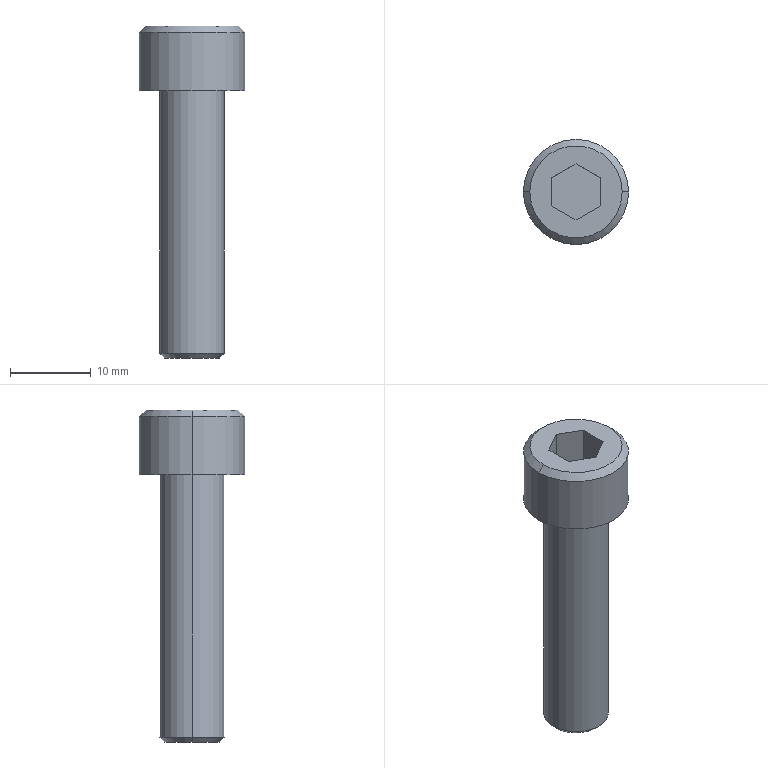Part | Creo | 1 solid | 18 faces | box 13 x 13 x 41 mm | volume 2554 mm3 | plane 10 | cylinder 4 | cone 4 | commonest cylinder face diameters 8 x2 13 x2
STEP:
#1=CARTESIAN_POINT('',(-49.837,-39.386,189.5));
#2=VERTEX_POINT('',#1);
#3=CARTESIAN_POINT('',(-62.837,-39.386,189.5));
#4=VERTEX_POINT('',#3);
#5=CARTESIAN_POINT('',(-56.337,-39.386,189.5));
#6=DIRECTION('',(0.,0.,-1.));
#7=DIRECTION('',(1.,0.,0.));
#8=AXIS2_PLACEMENT_3D('',#5,#6,#7);
#9=CIRCLE('',#8,6.5);
#10=EDGE_CURVE('',#2,#4,#9,.T.);
#11=ORIENTED_EDGE('',*,*,#10,.F.);
#12=CARTESIAN_POINT('',(-56.337,-39.386,189.5));
#13=DIRECTION('',(0.,0.,-1.));
#14=DIRECTION('',(-1.,0.,0.));
#15=AXIS2_PLACEMENT_3D('',#12,#13,#14);
#16=CIRCLE('',#15,6.5);
#17=EDGE_CURVE('',#4,#2,#16,.T.);
#18=ORIENTED_EDGE('',*,*,#17,.F.);
#19=EDGE_LOOP('',(#11,#18));
#20=FACE_OUTER_BOUND('',#19,.F.);
#21=CARTESIAN_POINT('',(-60.337,-39.386,189.5));
#22=VERTEX_POINT('',#21);
#23=CARTESIAN_POINT('',(-52.337,-39.386,189.5));
#24=VERTEX_POINT('',#23);
#25=CARTESIAN_POINT('',(-56.337,-39.386,189.5));
#26=DIRECTION('',(0.,0.,1.));
#27=DIRECTION('',(-1.,0.,0.));
#28=AXIS2_PLACEMENT_3D('',#25,#26,#27);
#29=CIRCLE('',#28,4.);
#30=EDGE_CURVE('',#22,#24,#29,.T.);
#31=ORIENTED_EDGE('',*,*,#30,.F.);
#32=CARTESIAN_POINT('',(-56.337,-39.386,189.5));
#33=DIRECTION('',(0.,0.,1.));
#34=DIRECTION('',(1.,0.,0.));
#35=AXIS2_PLACEMENT_3D('',#32,#33,#34);
#36=CIRCLE('',#35,4.);
#37=EDGE_CURVE('',#24,#22,#36,.T.);
#38=ORIENTED_EDGE('',*,*,#37,.F.);
#39=EDGE_LOOP('',(#31,#38));
#40=FACE_BOUND('',#39,.F.);
#41=CARTESIAN_POINT('',(-56.337,-39.386,189.5));
#42=DIRECTION('',(0.,0.,-1.));
#43=DIRECTION('',(-1.,0.,0.));
#44=AXIS2_PLACEMENT_3D('',#41,#42,#43);
#45=PLANE('',#44);
#46=ADVANCED_FACE('',(#20,#40),#45,.T.);
#47=CARTESIAN_POINT('',(-52.337,-39.386,157.1));
#48=VERTEX_POINT('',#47);
#49=CARTESIAN_POINT('',(-60.337,-39.386,157.1));
#50=VERTEX_POINT('',#49);
#51=CARTESIAN_POINT('',(-56.337,-39.386,157.1));
#52=DIRECTION('',(0.,0.,-1.));
#53=DIRECTION('',(1.,0.,0.));
#54=AXIS2_PLACEMENT_3D('',#51,#52,#53);
#55=CIRCLE('',#54,4.);
#56=EDGE_CURVE('',#48,#50,#55,.T.);
#57=ORIENTED_EDGE('',*,*,#56,.T.);
#58=CARTESIAN_POINT('',(-60.337,-39.386,189.5));
#59=DIRECTION('',(0.,0.,-1.));
#60=VECTOR('',#59,32.4);
#61=LINE('',#58,#60);
#62=EDGE_CURVE('',#22,#50,#61,.T.);
#63=ORIENTED_EDGE('',*,*,#62,.F.);
#64=ORIENTED_EDGE('',*,*,#30,.T.);
#65=CARTESIAN_POINT('',(-52.337,-39.386,189.5));
#66=DIRECTION('',(0.,0.,-1.));
#67=VECTOR('',#66,32.4);
#68=LINE('',#65,#67);
#69=EDGE_CURVE('',#24,#48,#68,.T.);
#70=ORIENTED_EDGE('',*,*,#69,.T.);
#71=EDGE_LOOP('',(#57,#63,#64,#70));
#72=FACE_OUTER_BOUND('',#71,.F.);
#73=CARTESIAN_POINT('',(-56.337,-39.386,210.5));
#74=DIRECTION('',(0.,0.,-1.));
#75=DIRECTION('',(-1.,0.,0.));
#76=AXIS2_PLACEMENT_3D('',#73,#74,#75);
#77=CYLINDRICAL_SURFACE('',#76,4.);
#78=ADVANCED_FACE('',(#72),#77,.T.);
#79=CARTESIAN_POINT('',(-52.937,-39.386,156.5));
#80=VERTEX_POINT('',#79);
#81=CARTESIAN_POINT('',(-59.737,-39.386,156.5));
#82=VERTEX_POINT('',#81);
#83=CARTESIAN_POINT('',(-56.337,-39.386,156.5));
#84=DIRECTION('',(0.,0.,-1.));
#85=DIRECTION('',(1.,0.,0.));
#86=AXIS2_PLACEMENT_3D('',#83,#84,#85);
#87=CIRCLE('',#86,3.4);
#88=EDGE_CURVE('',#80,#82,#87,.T.);
#89=ORIENTED_EDGE('',*,*,#88,.T.);
#90=CARTESIAN_POINT('',(-59.737,-39.386,156.5));
#91=DIRECTION('',(-0.7071,0.,0.7071));
#92=VECTOR('',#91,0.8485);
#93=LINE('',#90,#92);
#94=EDGE_CURVE('',#82,#50,#93,.T.);
#95=ORIENTED_EDGE('',*,*,#94,.T.);
#96=ORIENTED_EDGE('',*,*,#56,.F.);
#97=CARTESIAN_POINT('',(-52.937,-39.386,156.5));
#98=DIRECTION('',(0.7071,0.,0.7071));
#99=VECTOR('',#98,0.8485);
#100=LINE('',#97,#99);
#101=EDGE_CURVE('',#80,#48,#100,.T.);
#102=ORIENTED_EDGE('',*,*,#101,.F.);
#103=EDGE_LOOP('',(#89,#95,#96,#102));
#104=FACE_OUTER_BOUND('',#103,.F.);
#105=CARTESIAN_POINT('',(-56.337,-39.386,156.8));
#106=DIRECTION('',(0.,0.,1.));
#107=DIRECTION('',(1.,0.,0.));
#108=AXIS2_PLACEMENT_3D('',#105,#106,#107);
#109=CONICAL_SURFACE('',#108,3.7,45.);
#110=ADVANCED_FACE('',(#104),#109,.T.);
#111=CARTESIAN_POINT('',(-56.337,-39.386,156.5));
#112=DIRECTION('',(0.,0.,-1.));
#113=DIRECTION('',(-1.,0.,0.));
#114=AXIS2_PLACEMENT_3D('',#111,#112,#113);
#115=CIRCLE('',#114,3.4);
#116=EDGE_CURVE('',#82,#80,#115,.T.);
#117=ORIENTED_EDGE('',*,*,#116,.F.);
#118=ORIENTED_EDGE('',*,*,#88,.F.);
#119=EDGE_LOOP('',(#117,#118));
#120=FACE_OUTER_BOUND('',#119,.F.);
#121=CARTESIAN_POINT('',(-56.337,-39.386,156.5));
#122=DIRECTION('',(0.,0.,-1.));
#123=DIRECTION('',(-1.,0.,0.));
#124=AXIS2_PLACEMENT_3D('',#121,#122,#123);
#125=PLANE('',#124);
#126=ADVANCED_FACE('',(#120),#125,.T.);
#127=ORIENTED_EDGE('',*,*,#116,.T.);
#128=ORIENTED_EDGE('',*,*,#101,.T.);
#129=CARTESIAN_POINT('',(-56.337,-39.386,157.1));
#130=DIRECTION('',(0.,0.,-1.));
#131=DIRECTION('',(-1.,0.,0.));
#132=AXIS2_PLACEMENT_3D('',#129,#130,#131);
#133=CIRCLE('',#132,4.);
#134=EDGE_CURVE('',#50,#48,#133,.T.);
#135=ORIENTED_EDGE('',*,*,#134,.F.);
#136=ORIENTED_EDGE('',*,*,#94,.F.);
#137=EDGE_LOOP('',(#127,#128,#135,#136));
#138=FACE_OUTER_BOUND('',#137,.F.);
#139=CARTESIAN_POINT('',(-56.337,-39.386,156.8));
#140=DIRECTION('',(0.,0.,1.));
#141=DIRECTION('',(1.,0.,0.));
#142=AXIS2_PLACEMENT_3D('',#139,#140,#141);
#143=CONICAL_SURFACE('',#142,3.7,45.);
#144=ADVANCED_FACE('',(#138),#143,.T.);
#145=ORIENTED_EDGE('',*,*,#134,.T.);
#146=ORIENTED_EDGE('',*,*,#69,.F.);
#147=ORIENTED_EDGE('',*,*,#37,.T.);
#148=ORIENTED_EDGE('',*,*,#62,.T.);
#149=EDGE_LOOP('',(#145,#146,#147,#148));
#150=FACE_OUTER_BOUND('',#149,.F.);
#151=CARTESIAN_POINT('',(-56.337,-39.386,210.5));
#152=DIRECTION('',(0.,0.,-1.));
#153=DIRECTION('',(-1.,0.,0.));
#154=AXIS2_PLACEMENT_3D('',#151,#152,#153);
#155=CYLINDRICAL_SURFACE('',#154,4.);
#156=ADVANCED_FACE('',(#150),#155,.T.);
#157=CARTESIAN_POINT('',(-62.837,-39.386,196.7));
#158=VERTEX_POINT('',#157);
#159=CARTESIAN_POINT('',(-49.837,-39.386,196.7));
#160=VERTEX_POINT('',#159);
#161=CARTESIAN_POINT('',(-56.337,-39.386,196.7));
#162=DIRECTION('',(0.,0.,1.));
#163=DIRECTION('',(-1.,0.,0.));
#164=AXIS2_PLACEMENT_3D('',#161,#162,#163);
#165=CIRCLE('',#164,6.5);
#166=EDGE_CURVE('',#158,#160,#165,.T.);
#167=ORIENTED_EDGE('',*,*,#166,.T.);
#168=CARTESIAN_POINT('',(-49.837,-39.386,196.7));
#169=DIRECTION('',(0.,0.,-1.));
#170=VECTOR('',#169,7.2);
#171=LINE('',#168,#170);
#172=EDGE_CURVE('',#160,#2,#171,.T.);
#173=ORIENTED_EDGE('',*,*,#172,.T.);
#174=ORIENTED_EDGE('',*,*,#10,.T.);
#175=CARTESIAN_POINT('',(-62.837,-39.386,196.7));
#176=DIRECTION('',(0.,0.,-1.));
#177=VECTOR('',#176,7.2);
#178=LINE('',#175,#177);
#179=EDGE_CURVE('',#158,#4,#178,.T.);
#180=ORIENTED_EDGE('',*,*,#179,.F.);
#181=EDGE_LOOP('',(#167,#173,#174,#180));
#182=FACE_OUTER_BOUND('',#181,.F.);
#183=CARTESIAN_POINT('',(-56.337,-39.386,198.5));
#184=DIRECTION('',(0.,0.,-1.));
#185=DIRECTION('',(-1.,0.,0.));
#186=AXIS2_PLACEMENT_3D('',#183,#184,#185);
#187=CYLINDRICAL_SURFACE('',#186,6.5);
#188=ADVANCED_FACE('',(#182),#187,.T.);
#189=CARTESIAN_POINT('',(-62.037,-39.386,197.5));
#190=VERTEX_POINT('',#189);
#191=CARTESIAN_POINT('',(-50.637,-39.386,197.5));
#192=VERTEX_POINT('',#191);
#193=CARTESIAN_POINT('',(-56.337,-39.386,197.5));
#194=DIRECTION('',(0.,0.,1.));
#195=DIRECTION('',(-1.,0.,0.));
#196=AXIS2_PLACEMENT_3D('',#193,#194,#195);
#197=CIRCLE('',#196,5.7);
#198=EDGE_CURVE('',#190,#192,#197,.T.);
#199=ORIENTED_EDGE('',*,*,#198,.T.);
#200=CARTESIAN_POINT('',(-50.637,-39.386,197.5));
#201=DIRECTION('',(0.7071,0.,-0.7071));
#202=VECTOR('',#201,1.131);
#203=LINE('',#200,#202);
#204=EDGE_CURVE('',#192,#160,#203,.T.);
#205=ORIENTED_EDGE('',*,*,#204,.T.);
#206=ORIENTED_EDGE('',*,*,#166,.F.);
#207=CARTESIAN_POINT('',(-62.037,-39.386,197.5));
#208=DIRECTION('',(-0.7071,0.,-0.7071));
#209=VECTOR('',#208,1.131);
#210=LINE('',#207,#209);
#211=EDGE_CURVE('',#190,#158,#210,.T.);
#212=ORIENTED_EDGE('',*,*,#211,.F.);
#213=EDGE_LOOP('',(#199,#205,#206,#212));
#214=FACE_OUTER_BOUND('',#213,.F.);
#215=CARTESIAN_POINT('',(-56.337,-39.386,197.1));
#216=DIRECTION('',(0.,0.,-1.));
#217=DIRECTION('',(-1.,0.,0.));
#218=AXIS2_PLACEMENT_3D('',#215,#216,#217);
#219=CONICAL_SURFACE('',#218,6.1,45.);
#220=ADVANCED_FACE('',(#214),#219,.T.);
#221=ORIENTED_EDGE('',*,*,#198,.F.);
#222=CARTESIAN_POINT('',(-56.337,-39.386,197.5));
#223=DIRECTION('',(0.,0.,1.));
#224=DIRECTION('',(1.,0.,0.));
#225=AXIS2_PLACEMENT_3D('',#222,#223,#224);
#226=CIRCLE('',#225,5.7);
#227=EDGE_CURVE('',#192,#190,#226,.T.);
#228=ORIENTED_EDGE('',*,*,#227,.F.);
#229=EDGE_LOOP('',(#221,#228));
#230=FACE_OUTER_BOUND('',#229,.F.);
#231=CARTESIAN_POINT('',(-53.337,-41.118,197.5));
#232=VERTEX_POINT('',#231);
#233=CARTESIAN_POINT('',(-56.337,-42.85,197.5));
#234=VERTEX_POINT('',#233);
#235=CARTESIAN_POINT('',(-53.337,-41.118,197.5));
#236=DIRECTION('',(-0.866,-0.5,0.));
#237=VECTOR('',#236,3.464);
#238=LINE('',#235,#237);
#239=EDGE_CURVE('',#232,#234,#238,.T.);
#240=ORIENTED_EDGE('',*,*,#239,.F.);
#241=CARTESIAN_POINT('',(-53.337,-37.654,197.5));
#242=VERTEX_POINT('',#241);
#243=CARTESIAN_POINT('',(-53.337,-37.654,197.5));
#244=DIRECTION('',(0.,-1.,0.));
#245=VECTOR('',#244,3.464);
#246=LINE('',#243,#245);
#247=EDGE_CURVE('',#242,#232,#246,.T.);
#248=ORIENTED_EDGE('',*,*,#247,.F.);
#249=CARTESIAN_POINT('',(-56.337,-35.922,197.5));
#250=VERTEX_POINT('',#249);
#251=CARTESIAN_POINT('',(-56.337,-35.922,197.5));
#252=DIRECTION('',(0.866,-0.5,0.));
#253=VECTOR('',#252,3.464);
#254=LINE('',#251,#253);
#255=EDGE_CURVE('',#250,#242,#254,.T.);
#256=ORIENTED_EDGE('',*,*,#255,.F.);
#257=CARTESIAN_POINT('',(-59.337,-37.654,197.5));
#258=VERTEX_POINT('',#257);
#259=CARTESIAN_POINT('',(-59.337,-37.654,197.5));
#260=DIRECTION('',(0.866,0.5,0.));
#261=VECTOR('',#260,3.464);
#262=LINE('',#259,#261);
#263=EDGE_CURVE('',#258,#250,#262,.T.);
#264=ORIENTED_EDGE('',*,*,#263,.F.);
#265=CARTESIAN_POINT('',(-59.337,-41.118,197.5));
#266=VERTEX_POINT('',#265);
#267=CARTESIAN_POINT('',(-59.337,-41.118,197.5));
#268=DIRECTION('',(0.,1.,0.));
#269=VECTOR('',#268,3.464);
#270=LINE('',#267,#269);
#271=EDGE_CURVE('',#266,#258,#270,.T.);
#272=ORIENTED_EDGE('',*,*,#271,.F.);
#273=CARTESIAN_POINT('',(-56.337,-42.85,197.5));
#274=DIRECTION('',(-0.866,0.5,0.));
#275=VECTOR('',#274,3.464);
#276=LINE('',#273,#275);
#277=EDGE_CURVE('',#234,#266,#276,.T.);
#278=ORIENTED_EDGE('',*,*,#277,.F.);
#279=EDGE_LOOP('',(#240,#248,#256,#264,#272,#278));
#280=FACE_BOUND('',#279,.F.);
#281=CARTESIAN_POINT('',(-56.337,-39.386,197.5));
#282=DIRECTION('',(0.,0.,-1.));
#283=DIRECTION('',(-1.,0.,0.));
#284=AXIS2_PLACEMENT_3D('',#281,#282,#283);
#285=PLANE('',#284);
#286=ADVANCED_FACE('',(#230,#280),#285,.F.);
#287=ORIENTED_EDGE('',*,*,#227,.T.);
#288=ORIENTED_EDGE('',*,*,#211,.T.);
#289=CARTESIAN_POINT('',(-56.337,-39.386,196.7));
#290=DIRECTION('',(0.,0.,1.));
#291=DIRECTION('',(1.,0.,0.));
#292=AXIS2_PLACEMENT_3D('',#289,#290,#291);
#293=CIRCLE('',#292,6.5);
#294=EDGE_CURVE('',#160,#158,#293,.T.);
#295=ORIENTED_EDGE('',*,*,#294,.F.);
#296=ORIENTED_EDGE('',*,*,#204,.F.);
#297=EDGE_LOOP('',(#287,#288,#295,#296));
#298=FACE_OUTER_BOUND('',#297,.F.);
#299=CARTESIAN_POINT('',(-56.337,-39.386,197.1));
#300=DIRECTION('',(0.,0.,-1.));
#301=DIRECTION('',(-1.,0.,0.));
#302=AXIS2_PLACEMENT_3D('',#299,#300,#301);
#303=CONICAL_SURFACE('',#302,6.1,45.);
#304=ADVANCED_FACE('',(#298),#303,.T.);
#305=ORIENTED_EDGE('',*,*,#294,.T.);
#306=ORIENTED_EDGE('',*,*,#179,.T.);
#307=ORIENTED_EDGE('',*,*,#17,.T.);
#308=ORIENTED_EDGE('',*,*,#172,.F.);
#309=EDGE_LOOP('',(#305,#306,#307,#308));
#310=FACE_OUTER_BOUND('',#309,.F.);
#311=CARTESIAN_POINT('',(-56.337,-39.386,198.5));
#312=DIRECTION('',(0.,0.,-1.));
#313=DIRECTION('',(-1.,0.,0.));
#314=AXIS2_PLACEMENT_3D('',#311,#312,#313);
#315=CYLINDRICAL_SURFACE('',#314,6.5);
#316=ADVANCED_FACE('',(#310),#315,.T.);
#317=ORIENTED_EDGE('',*,*,#239,.T.);
#318=CARTESIAN_POINT('',(-56.337,-42.85,192.7));
#319=VERTEX_POINT('',#318);
#320=CARTESIAN_POINT('',(-56.337,-42.85,197.5));
#321=DIRECTION('',(0.,0.,-1.));
#322=VECTOR('',#321,4.8);
#323=LINE('',#320,#322);
#324=EDGE_CURVE('',#234,#319,#323,.T.);
#325=ORIENTED_EDGE('',*,*,#324,.T.);
#326=CARTESIAN_POINT('',(-53.337,-41.118,192.7));
#327=VERTEX_POINT('',#326);
#328=CARTESIAN_POINT('',(-56.337,-42.85,192.7));
#329=DIRECTION('',(0.866,0.5,0.));
#330=VECTOR('',#329,3.464);
#331=LINE('',#328,#330);
#332=EDGE_CURVE('',#319,#327,#331,.T.);
#333=ORIENTED_EDGE('',*,*,#332,.T.);
#334=CARTESIAN_POINT('',(-53.337,-41.118,197.5));
#335=DIRECTION('',(0.,0.,-1.));
#336=VECTOR('',#335,4.8);
#337=LINE('',#334,#336);
#338=EDGE_CURVE('',#232,#327,#337,.T.);
#339=ORIENTED_EDGE('',*,*,#338,.F.);
#340=EDGE_LOOP('',(#317,#325,#333,#339));
#341=FACE_OUTER_BOUND('',#340,.F.);
#342=CARTESIAN_POINT('',(-56.337,-42.85,192.7));
#343=DIRECTION('',(0.5,-0.866,0.));
#344=DIRECTION('',(0.866,0.5,0.));
#345=AXIS2_PLACEMENT_3D('',#342,#343,#344);
#346=PLANE('',#345);
#347=ADVANCED_FACE('',(#341),#346,.F.);
#348=ORIENTED_EDGE('',*,*,#277,.T.);
#349=CARTESIAN_POINT('',(-59.337,-41.118,192.7));
#350=VERTEX_POINT('',#349);
#351=CARTESIAN_POINT('',(-59.337,-41.118,197.5));
#352=DIRECTION('',(0.,0.,-1.));
#353=VECTOR('',#352,4.8);
#354=LINE('',#351,#353);
#355=EDGE_CURVE('',#266,#350,#354,.T.);
#356=ORIENTED_EDGE('',*,*,#355,.T.);
#357=CARTESIAN_POINT('',(-59.337,-41.118,192.7));
#358=DIRECTION('',(0.866,-0.5,0.));
#359=VECTOR('',#358,3.464);
#360=LINE('',#357,#359);
#361=EDGE_CURVE('',#350,#319,#360,.T.);
#362=ORIENTED_EDGE('',*,*,#361,.T.);
#363=ORIENTED_EDGE('',*,*,#324,.F.);
#364=EDGE_LOOP('',(#348,#356,#362,#363));
#365=FACE_OUTER_BOUND('',#364,.F.);
#366=CARTESIAN_POINT('',(-59.337,-41.118,192.7));
#367=DIRECTION('',(-0.5,-0.866,0.));
#368=DIRECTION('',(0.866,-0.5,0.));
#369=AXIS2_PLACEMENT_3D('',#366,#367,#368);
#370=PLANE('',#369);
#371=ADVANCED_FACE('',(#365),#370,.F.);
#372=ORIENTED_EDGE('',*,*,#271,.T.);
#373=CARTESIAN_POINT('',(-59.337,-37.654,192.7));
#374=VERTEX_POINT('',#373);
#375=CARTESIAN_POINT('',(-59.337,-37.654,197.5));
#376=DIRECTION('',(0.,0.,-1.));
#377=VECTOR('',#376,4.8);
#378=LINE('',#375,#377);
#379=EDGE_CURVE('',#258,#374,#378,.T.);
#380=ORIENTED_EDGE('',*,*,#379,.T.);
#381=CARTESIAN_POINT('',(-59.337,-41.118,192.7));
#382=DIRECTION('',(0.,1.,0.));
#383=VECTOR('',#382,3.464);
#384=LINE('',#381,#383);
#385=EDGE_CURVE('',#350,#374,#384,.T.);
#386=ORIENTED_EDGE('',*,*,#385,.F.);
#387=ORIENTED_EDGE('',*,*,#355,.F.);
#388=EDGE_LOOP('',(#372,#380,#386,#387));
#389=FACE_OUTER_BOUND('',#388,.F.);
#390=CARTESIAN_POINT('',(-59.337,-37.654,192.7));
#391=DIRECTION('',(-1.,0.,0.));
#392=DIRECTION('',(0.,0.,1.));
#393=AXIS2_PLACEMENT_3D('',#390,#391,#392);
#394=PLANE('',#393);
#395=ADVANCED_FACE('',(#389),#394,.F.);
#396=ORIENTED_EDGE('',*,*,#263,.T.);
#397=CARTESIAN_POINT('',(-56.337,-35.922,192.7));
#398=VERTEX_POINT('',#397);
#399=CARTESIAN_POINT('',(-56.337,-35.922,197.5));
#400=DIRECTION('',(0.,0.,-1.));
#401=VECTOR('',#400,4.8);
#402=LINE('',#399,#401);
#403=EDGE_CURVE('',#250,#398,#402,.T.);
#404=ORIENTED_EDGE('',*,*,#403,.T.);
#405=CARTESIAN_POINT('',(-56.337,-35.922,192.7));
#406=DIRECTION('',(-0.866,-0.5,0.));
#407=VECTOR('',#406,3.464);
#408=LINE('',#405,#407);
#409=EDGE_CURVE('',#398,#374,#408,.T.);
#410=ORIENTED_EDGE('',*,*,#409,.T.);
#411=ORIENTED_EDGE('',*,*,#379,.F.);
#412=EDGE_LOOP('',(#396,#404,#410,#411));
#413=FACE_OUTER_BOUND('',#412,.F.);
#414=CARTESIAN_POINT('',(-56.337,-35.922,192.7));
#415=DIRECTION('',(-0.5,0.866,0.));
#416=DIRECTION('',(-0.866,-0.5,0.));
#417=AXIS2_PLACEMENT_3D('',#414,#415,#416);
#418=PLANE('',#417);
#419=ADVANCED_FACE('',(#413),#418,.F.);
#420=ORIENTED_EDGE('',*,*,#255,.T.);
#421=CARTESIAN_POINT('',(-53.337,-37.654,192.7));
#422=VERTEX_POINT('',#421);
#423=CARTESIAN_POINT('',(-53.337,-37.654,197.5));
#424=DIRECTION('',(0.,0.,-1.));
#425=VECTOR('',#424,4.8);
#426=LINE('',#423,#425);
#427=EDGE_CURVE('',#242,#422,#426,.T.);
#428=ORIENTED_EDGE('',*,*,#427,.T.);
#429=CARTESIAN_POINT('',(-53.337,-37.654,192.7));
#430=DIRECTION('',(-0.866,0.5,0.));
#431=VECTOR('',#430,3.464);
#432=LINE('',#429,#431);
#433=EDGE_CURVE('',#422,#398,#432,.T.);
#434=ORIENTED_EDGE('',*,*,#433,.T.);
#435=ORIENTED_EDGE('',*,*,#403,.F.);
#436=EDGE_LOOP('',(#420,#428,#434,#435));
#437=FACE_OUTER_BOUND('',#436,.F.);
#438=CARTESIAN_POINT('',(-53.337,-37.654,192.7));
#439=DIRECTION('',(0.5,0.866,0.));
#440=DIRECTION('',(-0.866,0.5,0.));
#441=AXIS2_PLACEMENT_3D('',#438,#439,#440);
#442=PLANE('',#441);
#443=ADVANCED_FACE('',(#437),#442,.F.);
#444=ORIENTED_EDGE('',*,*,#247,.T.);
#445=ORIENTED_EDGE('',*,*,#338,.T.);
#446=CARTESIAN_POINT('',(-53.337,-37.654,192.7));
#447=DIRECTION('',(0.,-1.,0.));
#448=VECTOR('',#447,3.464);
#449=LINE('',#446,#448);
#450=EDGE_CURVE('',#422,#327,#449,.T.);
#451=ORIENTED_EDGE('',*,*,#450,.F.);
#452=ORIENTED_EDGE('',*,*,#427,.F.);
#453=EDGE_LOOP('',(#444,#445,#451,#452));
#454=FACE_OUTER_BOUND('',#453,.F.);
#455=CARTESIAN_POINT('',(-53.337,-41.118,192.7));
#456=DIRECTION('',(1.,0.,0.));
#457=DIRECTION('',(0.,0.,-1.));
#458=AXIS2_PLACEMENT_3D('',#455,#456,#457);
#459=PLANE('',#458);
#460=ADVANCED_FACE('',(#454),#459,.F.);
#461=ORIENTED_EDGE('',*,*,#361,.F.);
#462=ORIENTED_EDGE('',*,*,#385,.T.);
#463=ORIENTED_EDGE('',*,*,#409,.F.);
#464=ORIENTED_EDGE('',*,*,#433,.F.);
#465=ORIENTED_EDGE('',*,*,#450,.T.);
#466=ORIENTED_EDGE('',*,*,#332,.F.);
#467=EDGE_LOOP('',(#461,#462,#463,#464,#465,#466));
#468=FACE_OUTER_BOUND('',#467,.F.);
#469=CARTESIAN_POINT('',(-56.337,-42.85,192.7));
#470=DIRECTION('',(0.,0.,1.));
#471=DIRECTION('',(1.,0.,0.));
#472=AXIS2_PLACEMENT_3D('',#469,#470,#471);
#473=PLANE('',#472);
#474=ADVANCED_FACE('',(#468),#473,.T.);
#475=CLOSED_SHELL('',(#46,#78,#110,#126,#144,#156,#188,#220,#286,#304,#316,#347,#371,#395,#419,#443,#460,#474));
#476=MANIFOLD_SOLID_BREP('',#475);
#477=(LENGTH_UNIT()NAMED_UNIT(*)SI_UNIT(.MILLI.,.METRE.));
#478=UNCERTAINTY_MEASURE_WITH_UNIT(LENGTH_MEASURE(0.004494),#477,'','');
#479=(NAMED_UNIT(*)PLANE_ANGLE_UNIT()SI_UNIT($,.RADIAN.));
#480=PLANE_ANGLE_MEASURE_WITH_UNIT(PLANE_ANGLE_MEASURE(0.01745),#479);
#481=(CONVERSION_BASED_UNIT('DEGREE',#480)NAMED_UNIT(*)PLANE_ANGLE_UNIT());
#482=(NAMED_UNIT(*)SI_UNIT($,.STERADIAN.)SOLID_ANGLE_UNIT());
#483=(GEOMETRIC_REPRESENTATION_CONTEXT(3)GLOBAL_UNCERTAINTY_ASSIGNED_CONTEXT((#478))GLOBAL_UNIT_ASSIGNED_CONTEXT((#477,#481,#482))REPRESENTATION_CONTEXT('',''));
#484=ADVANCED_BREP_SHAPE_REPRESENTATION('',(#476),#483);